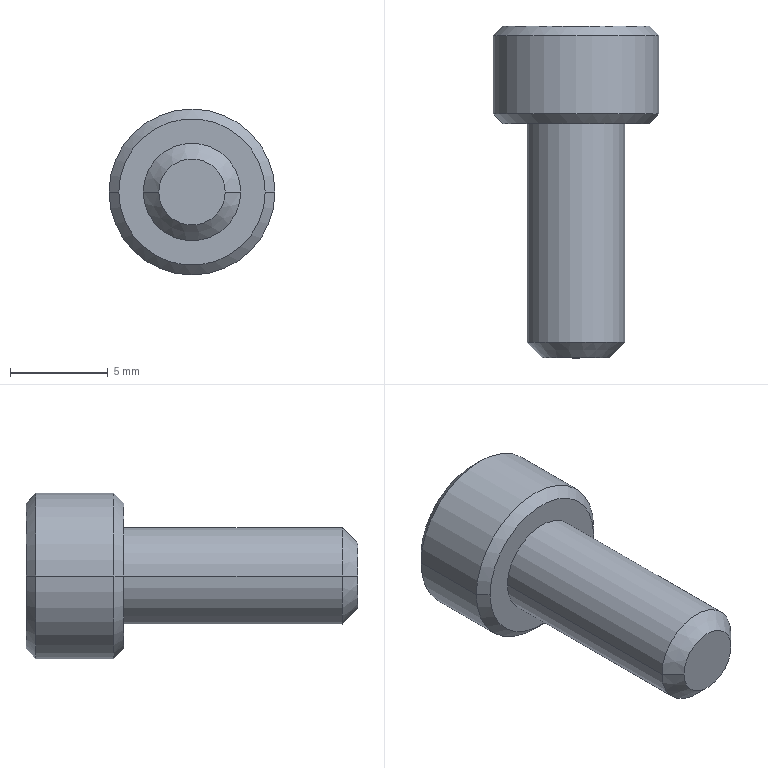Part | STEP file | BB62-M5-12L-13 | 1 solid | 27 faces | box 8.5 x 17 x 8.5 mm | volume 467.118 mm3 | plane 15 | cone 8 | cylinder 4 | commonest cylinder face diameters 5 x2 8.5 x2
STEP:
#1=CARTESIAN_POINT('',(0.,1.178,0.));
#2=VERTEX_POINT('',#1);
#3=CARTESIAN_POINT('',(2.29,2.5,0.));
#4=VERTEX_POINT('',#3);
#5=CARTESIAN_POINT('',(0.,1.178,0.));
#6=DIRECTION('',(0.866,0.5,0.));
#7=VECTOR('',#6,1000.);
#8=LINE('',#5,#7);
#9=EDGE_CURVE('',#2,#4,#8,.T.);
#10=ORIENTED_EDGE('',*,*,#9,.F.);
#11=CARTESIAN_POINT('',(-2.29,2.5,0.));
#12=VERTEX_POINT('',#11);
#13=CARTESIAN_POINT('',(0.,1.178,0.));
#14=DIRECTION('',(-0.866,0.5,0.));
#15=VECTOR('',#14,1000.);
#16=LINE('',#13,#15);
#17=EDGE_CURVE('',#2,#12,#16,.T.);
#18=ORIENTED_EDGE('',*,*,#17,.T.);
#19=CARTESIAN_POINT('',(-1.983,2.5,1.145));
#20=VERTEX_POINT('',#19);
#21=CARTESIAN_POINT('',(0.,2.5,0.));
#22=DIRECTION('',(0.,-1.,0.));
#23=DIRECTION('',(-1.,0.,0.));
#24=AXIS2_PLACEMENT_3D('',#21,#22,#23);
#25=CIRCLE('',#24,2.29);
#26=EDGE_CURVE('',#20,#12,#25,.T.);
#27=ORIENTED_EDGE('',*,*,#26,.F.);
#28=CARTESIAN_POINT('',(0.,2.5,2.29));
#29=VERTEX_POINT('',#28);
#30=CARTESIAN_POINT('',(0.,2.5,0.));
#31=DIRECTION('',(0.,-1.,0.));
#32=DIRECTION('',(-1.,0.,0.));
#33=AXIS2_PLACEMENT_3D('',#30,#31,#32);
#34=CIRCLE('',#33,2.29);
#35=EDGE_CURVE('',#29,#20,#34,.T.);
#36=ORIENTED_EDGE('',*,*,#35,.F.);
#37=CARTESIAN_POINT('',(1.983,2.5,1.145));
#38=VERTEX_POINT('',#37);
#39=CARTESIAN_POINT('',(0.,2.5,0.));
#40=DIRECTION('',(0.,-1.,0.));
#41=DIRECTION('',(-1.,0.,0.));
#42=AXIS2_PLACEMENT_3D('',#39,#40,#41);
#43=CIRCLE('',#42,2.29);
#44=EDGE_CURVE('',#38,#29,#43,.T.);
#45=ORIENTED_EDGE('',*,*,#44,.F.);
#46=CARTESIAN_POINT('',(0.,2.5,0.));
#47=DIRECTION('',(0.,-1.,0.));
#48=DIRECTION('',(-1.,0.,0.));
#49=AXIS2_PLACEMENT_3D('',#46,#47,#48);
#50=CIRCLE('',#49,2.29);
#51=EDGE_CURVE('',#4,#38,#50,.T.);
#52=ORIENTED_EDGE('',*,*,#51,.F.);
#53=EDGE_LOOP('',(#10,#18,#27,#36,#45,#52));
#54=FACE_OUTER_BOUND('',#53,.T.);
#55=CARTESIAN_POINT('',(0.,1001.178,0.));
#56=DIRECTION('',(0.,1.,0.));
#57=DIRECTION('',(1.,0.,0.));
#58=AXIS2_PLACEMENT_3D('',#55,#56,#57);
#59=CONICAL_SURFACE('',#58,1732.051,1.047);
#60=ADVANCED_FACE('',(#54),#59,.F.);
#61=CARTESIAN_POINT('',(1.7,-12.,0.));
#62=VERTEX_POINT('',#61);
#63=CARTESIAN_POINT('',(-1.7,-12.,0.));
#64=VERTEX_POINT('',#63);
#65=CARTESIAN_POINT('',(0.,-12.,0.));
#66=DIRECTION('',(0.,1.,0.));
#67=DIRECTION('',(1.,0.,0.));
#68=AXIS2_PLACEMENT_3D('',#65,#66,#67);
#69=CIRCLE('',#68,1.7);
#70=EDGE_CURVE('',#62,#64,#69,.T.);
#71=ORIENTED_EDGE('',*,*,#70,.T.);
#72=CARTESIAN_POINT('',(-2.5,-11.2,0.));
#73=VERTEX_POINT('',#72);
#74=CARTESIAN_POINT('',(-1.7,-12.,0.));
#75=DIRECTION('',(-0.7071,0.7071,0.));
#76=VECTOR('',#75,1000.);
#77=LINE('',#74,#76);
#78=EDGE_CURVE('',#64,#73,#77,.T.);
#79=ORIENTED_EDGE('',*,*,#78,.T.);
#80=CARTESIAN_POINT('',(2.5,-11.2,0.));
#81=VERTEX_POINT('',#80);
#82=CARTESIAN_POINT('',(0.,-11.2,0.));
#83=DIRECTION('',(0.,-1.,0.));
#84=DIRECTION('',(-1.,0.,0.));
#85=AXIS2_PLACEMENT_3D('',#82,#83,#84);
#86=CIRCLE('',#85,2.5);
#87=EDGE_CURVE('',#73,#81,#86,.T.);
#88=ORIENTED_EDGE('',*,*,#87,.T.);
#89=CARTESIAN_POINT('',(1.7,-12.,0.));
#90=DIRECTION('',(0.7071,0.7071,0.));
#91=VECTOR('',#90,1000.);
#92=LINE('',#89,#91);
#93=EDGE_CURVE('',#62,#81,#92,.T.);
#94=ORIENTED_EDGE('',*,*,#93,.F.);
#95=EDGE_LOOP('',(#71,#79,#88,#94));
#96=FACE_OUTER_BOUND('',#95,.T.);
#97=CARTESIAN_POINT('',(0.,-12.,0.));
#98=DIRECTION('',(0.,1.,0.));
#99=DIRECTION('',(1.,0.,0.));
#100=AXIS2_PLACEMENT_3D('',#97,#98,#99);
#101=CONICAL_SURFACE('',#100,1.7,0.7854);
#102=ADVANCED_FACE('',(#96),#101,.T.);
#103=ORIENTED_EDGE('',*,*,#87,.F.);
#104=CARTESIAN_POINT('',(-2.5,0.,0.));
#105=VERTEX_POINT('',#104);
#106=CARTESIAN_POINT('',(-2.5,-11.2,0.));
#107=DIRECTION('',(0.,1.,0.));
#108=VECTOR('',#107,1000.);
#109=LINE('',#106,#108);
#110=EDGE_CURVE('',#73,#105,#109,.T.);
#111=ORIENTED_EDGE('',*,*,#110,.T.);
#112=CARTESIAN_POINT('',(2.5,0.,0.));
#113=VERTEX_POINT('',#112);
#114=CARTESIAN_POINT('',(0.,0.,0.));
#115=DIRECTION('',(0.,-1.,0.));
#116=DIRECTION('',(-1.,0.,0.));
#117=AXIS2_PLACEMENT_3D('',#114,#115,#116);
#118=CIRCLE('',#117,2.5);
#119=EDGE_CURVE('',#105,#113,#118,.T.);
#120=ORIENTED_EDGE('',*,*,#119,.T.);
#121=CARTESIAN_POINT('',(2.5,-11.2,0.));
#122=DIRECTION('',(0.,1.,0.));
#123=VECTOR('',#122,1000.);
#124=LINE('',#121,#123);
#125=EDGE_CURVE('',#81,#113,#124,.T.);
#126=ORIENTED_EDGE('',*,*,#125,.F.);
#127=EDGE_LOOP('',(#103,#111,#120,#126));
#128=FACE_OUTER_BOUND('',#127,.T.);
#129=CARTESIAN_POINT('',(0.,-11.2,0.));
#130=DIRECTION('',(0.,1.,0.));
#131=DIRECTION('',(1.,0.,0.));
#132=AXIS2_PLACEMENT_3D('',#129,#130,#131);
#133=CYLINDRICAL_SURFACE('',#132,2.5);
#134=ADVANCED_FACE('',(#128),#133,.T.);
#135=CARTESIAN_POINT('',(-3.75,5.,0.));
#136=VERTEX_POINT('',#135);
#137=CARTESIAN_POINT('',(3.75,5.,0.));
#138=VERTEX_POINT('',#137);
#139=CARTESIAN_POINT('',(0.,5.,0.));
#140=DIRECTION('',(0.,-1.,0.));
#141=DIRECTION('',(-1.,0.,0.));
#142=AXIS2_PLACEMENT_3D('',#139,#140,#141);
#143=CIRCLE('',#142,3.75);
#144=EDGE_CURVE('',#136,#138,#143,.T.);
#145=ORIENTED_EDGE('',*,*,#144,.T.);
#146=CARTESIAN_POINT('',(4.25,4.5,0.));
#147=VERTEX_POINT('',#146);
#148=CARTESIAN_POINT('',(4.25,4.5,0.));
#149=DIRECTION('',(0.7071,-0.7071,0.));
#150=VECTOR('',#149,1000.);
#151=LINE('',#148,#150);
#152=EDGE_CURVE('',#138,#147,#151,.T.);
#153=ORIENTED_EDGE('',*,*,#152,.T.);
#154=CARTESIAN_POINT('',(-4.25,4.5,0.));
#155=VERTEX_POINT('',#154);
#156=CARTESIAN_POINT('',(0.,4.5,0.));
#157=DIRECTION('',(0.,-1.,0.));
#158=DIRECTION('',(-1.,0.,0.));
#159=AXIS2_PLACEMENT_3D('',#156,#157,#158);
#160=CIRCLE('',#159,4.25);
#161=EDGE_CURVE('',#155,#147,#160,.T.);
#162=ORIENTED_EDGE('',*,*,#161,.F.);
#163=CARTESIAN_POINT('',(-4.25,4.5,0.));
#164=DIRECTION('',(-0.7071,-0.7071,0.));
#165=VECTOR('',#164,1000.);
#166=LINE('',#163,#165);
#167=EDGE_CURVE('',#136,#155,#166,.T.);
#168=ORIENTED_EDGE('',*,*,#167,.F.);
#169=EDGE_LOOP('',(#145,#153,#162,#168));
#170=FACE_OUTER_BOUND('',#169,.T.);
#171=CARTESIAN_POINT('',(0.,4.5,0.));
#172=DIRECTION('',(0.,-1.,0.));
#173=DIRECTION('',(-1.,0.,0.));
#174=AXIS2_PLACEMENT_3D('',#171,#172,#173);
#175=CONICAL_SURFACE('',#174,4.25,0.7854);
#176=ADVANCED_FACE('',(#170),#175,.T.);
#177=ORIENTED_EDGE('',*,*,#161,.T.);
#178=CARTESIAN_POINT('',(4.25,0.5,0.));
#179=VERTEX_POINT('',#178);
#180=CARTESIAN_POINT('',(4.25,1.62,0.));
#181=DIRECTION('',(0.,-1.,0.));
#182=VECTOR('',#181,1000.);
#183=LINE('',#180,#182);
#184=EDGE_CURVE('',#147,#179,#183,.T.);
#185=ORIENTED_EDGE('',*,*,#184,.T.);
#186=CARTESIAN_POINT('',(-4.25,0.5,0.));
#187=VERTEX_POINT('',#186);
#188=CARTESIAN_POINT('',(0.,0.5,0.));
#189=DIRECTION('',(0.,-1.,0.));
#190=DIRECTION('',(-1.,0.,0.));
#191=AXIS2_PLACEMENT_3D('',#188,#189,#190);
#192=CIRCLE('',#191,4.25);
#193=EDGE_CURVE('',#187,#179,#192,.T.);
#194=ORIENTED_EDGE('',*,*,#193,.F.);
#195=CARTESIAN_POINT('',(-4.25,1.62,0.));
#196=DIRECTION('',(0.,-1.,0.));
#197=VECTOR('',#196,1000.);
#198=LINE('',#195,#197);
#199=EDGE_CURVE('',#155,#187,#198,.T.);
#200=ORIENTED_EDGE('',*,*,#199,.F.);
#201=EDGE_LOOP('',(#177,#185,#194,#200));
#202=FACE_OUTER_BOUND('',#201,.T.);
#203=CARTESIAN_POINT('',(0.,1.62,0.));
#204=DIRECTION('',(0.,-1.,0.));
#205=DIRECTION('',(-1.,0.,0.));
#206=AXIS2_PLACEMENT_3D('',#203,#204,#205);
#207=CYLINDRICAL_SURFACE('',#206,4.25);
#208=ADVANCED_FACE('',(#202),#207,.T.);
#209=CARTESIAN_POINT('',(-3.75,0.,0.));
#210=VERTEX_POINT('',#209);
#211=CARTESIAN_POINT('',(3.75,0.,0.));
#212=VERTEX_POINT('',#211);
#213=CARTESIAN_POINT('',(0.,0.,0.));
#214=DIRECTION('',(0.,-1.,0.));
#215=DIRECTION('',(-1.,0.,0.));
#216=AXIS2_PLACEMENT_3D('',#213,#214,#215);
#217=CIRCLE('',#216,3.75);
#218=EDGE_CURVE('',#210,#212,#217,.T.);
#219=ORIENTED_EDGE('',*,*,#218,.F.);
#220=CARTESIAN_POINT('',(-3.75,0.,0.));
#221=DIRECTION('',(-0.7071,0.7071,0.));
#222=VECTOR('',#221,1000.);
#223=LINE('',#220,#222);
#224=EDGE_CURVE('',#210,#187,#223,.T.);
#225=ORIENTED_EDGE('',*,*,#224,.T.);
#226=ORIENTED_EDGE('',*,*,#193,.T.);
#227=CARTESIAN_POINT('',(3.75,0.,0.));
#228=DIRECTION('',(0.7071,0.7071,0.));
#229=VECTOR('',#228,1000.);
#230=LINE('',#227,#229);
#231=EDGE_CURVE('',#212,#179,#230,.T.);
#232=ORIENTED_EDGE('',*,*,#231,.F.);
#233=EDGE_LOOP('',(#219,#225,#226,#232));
#234=FACE_OUTER_BOUND('',#233,.T.);
#235=CARTESIAN_POINT('',(0.,0.,0.));
#236=DIRECTION('',(0.,1.,0.));
#237=DIRECTION('',(1.,0.,0.));
#238=AXIS2_PLACEMENT_3D('',#235,#236,#237);
#239=CONICAL_SURFACE('',#238,3.75,0.7854);
#240=ADVANCED_FACE('',(#234),#239,.T.);
#241=ORIENTED_EDGE('',*,*,#144,.F.);
#242=CARTESIAN_POINT('',(0.,5.,0.));
#243=DIRECTION('',(0.,-1.,0.));
#244=DIRECTION('',(-1.,0.,0.));
#245=AXIS2_PLACEMENT_3D('',#242,#243,#244);
#246=CIRCLE('',#245,3.75);
#247=EDGE_CURVE('',#138,#136,#246,.T.);
#248=ORIENTED_EDGE('',*,*,#247,.F.);
#249=EDGE_LOOP('',(#241,#248));
#250=FACE_OUTER_BOUND('',#249,.T.);
#251=CARTESIAN_POINT('',(0.,5.,-2.29));
#252=VERTEX_POINT('',#251);
#253=CARTESIAN_POINT('',(-1.983,5.,-1.145));
#254=VERTEX_POINT('',#253);
#255=CARTESIAN_POINT('',(0.,5.,-2.29));
#256=DIRECTION('',(-0.866,0.,0.5));
#257=VECTOR('',#256,1000.);
#258=LINE('',#255,#257);
#259=EDGE_CURVE('',#252,#254,#258,.T.);
#260=ORIENTED_EDGE('',*,*,#259,.F.);
#261=CARTESIAN_POINT('',(1.983,5.,-1.145));
#262=VERTEX_POINT('',#261);
#263=CARTESIAN_POINT('',(1.983,5.,-1.145));
#264=DIRECTION('',(-0.866,0.,-0.5));
#265=VECTOR('',#264,1000.);
#266=LINE('',#263,#265);
#267=EDGE_CURVE('',#262,#252,#266,.T.);
#268=ORIENTED_EDGE('',*,*,#267,.F.);
#269=CARTESIAN_POINT('',(1.983,5.,1.145));
#270=VERTEX_POINT('',#269);
#271=CARTESIAN_POINT('',(1.983,5.,1.145));
#272=DIRECTION('',(0.,0.,-1.));
#273=VECTOR('',#272,1000.);
#274=LINE('',#271,#273);
#275=EDGE_CURVE('',#270,#262,#274,.T.);
#276=ORIENTED_EDGE('',*,*,#275,.F.);
#277=CARTESIAN_POINT('',(0.,5.,2.29));
#278=VERTEX_POINT('',#277);
#279=CARTESIAN_POINT('',(0.,5.,2.29));
#280=DIRECTION('',(0.866,0.,-0.5));
#281=VECTOR('',#280,1000.);
#282=LINE('',#279,#281);
#283=EDGE_CURVE('',#278,#270,#282,.T.);
#284=ORIENTED_EDGE('',*,*,#283,.F.);
#285=CARTESIAN_POINT('',(-1.983,5.,1.145));
#286=VERTEX_POINT('',#285);
#287=CARTESIAN_POINT('',(-1.983,5.,1.145));
#288=DIRECTION('',(0.866,0.,0.5));
#289=VECTOR('',#288,1000.);
#290=LINE('',#287,#289);
#291=EDGE_CURVE('',#286,#278,#290,.T.);
#292=ORIENTED_EDGE('',*,*,#291,.F.);
#293=CARTESIAN_POINT('',(-1.983,5.,-1.145));
#294=DIRECTION('',(0.,0.,1.));
#295=VECTOR('',#294,1000.);
#296=LINE('',#293,#295);
#297=EDGE_CURVE('',#254,#286,#296,.T.);
#298=ORIENTED_EDGE('',*,*,#297,.F.);
#299=EDGE_LOOP('',(#260,#268,#276,#284,#292,#298));
#300=FACE_BOUND('',#299,.T.);
#301=CARTESIAN_POINT('',(3.75,5.,0.));
#302=DIRECTION('',(0.,1.,0.));
#303=DIRECTION('',(1.,0.,0.));
#304=AXIS2_PLACEMENT_3D('',#301,#302,#303);
#305=PLANE('',#304);
#306=ADVANCED_FACE('',(#250,#300),#305,.T.);
#307=CARTESIAN_POINT('',(0.,0.,0.));
#308=DIRECTION('',(0.,-1.,0.));
#309=DIRECTION('',(-1.,0.,0.));
#310=AXIS2_PLACEMENT_3D('',#307,#308,#309);
#311=CIRCLE('',#310,2.5);
#312=EDGE_CURVE('',#113,#105,#311,.T.);
#313=ORIENTED_EDGE('',*,*,#312,.F.);
#314=ORIENTED_EDGE('',*,*,#119,.F.);
#315=EDGE_LOOP('',(#313,#314));
#316=FACE_BOUND('',#315,.T.);
#317=CARTESIAN_POINT('',(0.,0.,0.));
#318=DIRECTION('',(0.,-1.,0.));
#319=DIRECTION('',(-1.,0.,0.));
#320=AXIS2_PLACEMENT_3D('',#317,#318,#319);
#321=CIRCLE('',#320,3.75);
#322=EDGE_CURVE('',#212,#210,#321,.T.);
#323=ORIENTED_EDGE('',*,*,#322,.T.);
#324=ORIENTED_EDGE('',*,*,#218,.T.);
#325=EDGE_LOOP('',(#323,#324));
#326=FACE_OUTER_BOUND('',#325,.T.);
#327=CARTESIAN_POINT('',(0.,0.,0.));
#328=DIRECTION('',(0.,-1.,0.));
#329=DIRECTION('',(-1.,0.,0.));
#330=AXIS2_PLACEMENT_3D('',#327,#328,#329);
#331=PLANE('',#330);
#332=ADVANCED_FACE('',(#316,#326),#331,.T.);
#333=ORIENTED_EDGE('',*,*,#224,.F.);
#334=ORIENTED_EDGE('',*,*,#322,.F.);
#335=ORIENTED_EDGE('',*,*,#231,.T.);
#336=CARTESIAN_POINT('',(0.,0.5,0.));
#337=DIRECTION('',(0.,-1.,0.));
#338=DIRECTION('',(-1.,0.,0.));
#339=AXIS2_PLACEMENT_3D('',#336,#337,#338);
#340=CIRCLE('',#339,4.25);
#341=EDGE_CURVE('',#179,#187,#340,.T.);
#342=ORIENTED_EDGE('',*,*,#341,.T.);
#343=EDGE_LOOP('',(#333,#334,#335,#342));
#344=FACE_OUTER_BOUND('',#343,.T.);
#345=CARTESIAN_POINT('',(0.,0.,0.));
#346=DIRECTION('',(0.,1.,0.));
#347=DIRECTION('',(1.,0.,0.));
#348=AXIS2_PLACEMENT_3D('',#345,#346,#347);
#349=CONICAL_SURFACE('',#348,3.75,0.7854);
#350=ADVANCED_FACE('',(#344),#349,.T.);
#351=ORIENTED_EDGE('',*,*,#184,.F.);
#352=CARTESIAN_POINT('',(0.,4.5,0.));
#353=DIRECTION('',(0.,-1.,0.));
#354=DIRECTION('',(-1.,0.,0.));
#355=AXIS2_PLACEMENT_3D('',#352,#353,#354);
#356=CIRCLE('',#355,4.25);
#357=EDGE_CURVE('',#147,#155,#356,.T.);
#358=ORIENTED_EDGE('',*,*,#357,.T.);
#359=ORIENTED_EDGE('',*,*,#199,.T.);
#360=ORIENTED_EDGE('',*,*,#341,.F.);
#361=EDGE_LOOP('',(#351,#358,#359,#360));
#362=FACE_OUTER_BOUND('',#361,.T.);
#363=CARTESIAN_POINT('',(0.,1.62,0.));
#364=DIRECTION('',(0.,-1.,0.));
#365=DIRECTION('',(-1.,0.,0.));
#366=AXIS2_PLACEMENT_3D('',#363,#364,#365);
#367=CYLINDRICAL_SURFACE('',#366,4.25);
#368=ADVANCED_FACE('',(#362),#367,.T.);
#369=ORIENTED_EDGE('',*,*,#152,.F.);
#370=ORIENTED_EDGE('',*,*,#247,.T.);
#371=ORIENTED_EDGE('',*,*,#167,.T.);
#372=ORIENTED_EDGE('',*,*,#357,.F.);
#373=EDGE_LOOP('',(#369,#370,#371,#372));
#374=FACE_OUTER_BOUND('',#373,.T.);
#375=CARTESIAN_POINT('',(0.,4.5,0.));
#376=DIRECTION('',(0.,-1.,0.));
#377=DIRECTION('',(-1.,0.,0.));
#378=AXIS2_PLACEMENT_3D('',#375,#376,#377);
#379=CONICAL_SURFACE('',#378,4.25,0.7854);
#380=ADVANCED_FACE('',(#374),#379,.T.);
#381=ORIENTED_EDGE('',*,*,#110,.F.);
#382=CARTESIAN_POINT('',(0.,-11.2,0.));
#383=DIRECTION('',(0.,-1.,0.));
#384=DIRECTION('',(-1.,0.,0.));
#385=AXIS2_PLACEMENT_3D('',#382,#383,#384);
#386=CIRCLE('',#385,2.5);
#387=EDGE_CURVE('',#81,#73,#386,.T.);
#388=ORIENTED_EDGE('',*,*,#387,.F.);
#389=ORIENTED_EDGE('',*,*,#125,.T.);
#390=ORIENTED_EDGE('',*,*,#312,.T.);
#391=EDGE_LOOP('',(#381,#388,#389,#390));
#392=FACE_OUTER_BOUND('',#391,.T.);
#393=CARTESIAN_POINT('',(0.,-11.2,0.));
#394=DIRECTION('',(0.,1.,0.));
#395=DIRECTION('',(1.,0.,0.));
#396=AXIS2_PLACEMENT_3D('',#393,#394,#395);
#397=CYLINDRICAL_SURFACE('',#396,2.5);
#398=ADVANCED_FACE('',(#392),#397,.T.);
#399=ORIENTED_EDGE('',*,*,#70,.F.);
#400=CARTESIAN_POINT('',(0.,-12.,0.));
#401=DIRECTION('',(0.,1.,0.));
#402=DIRECTION('',(1.,0.,0.));
#403=AXIS2_PLACEMENT_3D('',#400,#401,#402);
#404=CIRCLE('',#403,1.7);
#405=EDGE_CURVE('',#64,#62,#404,.T.);
#406=ORIENTED_EDGE('',*,*,#405,.F.);
#407=EDGE_LOOP('',(#399,#406));
#408=FACE_OUTER_BOUND('',#407,.T.);
#409=CARTESIAN_POINT('',(0.,-12.,0.));
#410=DIRECTION('',(0.,-1.,0.));
#411=DIRECTION('',(-1.,0.,0.));
#412=AXIS2_PLACEMENT_3D('',#409,#410,#411);
#413=PLANE('',#412);
#414=ADVANCED_FACE('',(#408),#413,.T.);
#415=ORIENTED_EDGE('',*,*,#78,.F.);
#416=ORIENTED_EDGE('',*,*,#405,.T.);
#417=ORIENTED_EDGE('',*,*,#93,.T.);
#418=ORIENTED_EDGE('',*,*,#387,.T.);
#419=EDGE_LOOP('',(#415,#416,#417,#418));
#420=FACE_OUTER_BOUND('',#419,.T.);
#421=CARTESIAN_POINT('',(0.,-12.,0.));
#422=DIRECTION('',(0.,1.,0.));
#423=DIRECTION('',(1.,0.,0.));
#424=AXIS2_PLACEMENT_3D('',#421,#422,#423);
#425=CONICAL_SURFACE('',#424,1.7,0.7854);
#426=ADVANCED_FACE('',(#420),#425,.T.);
#427=CARTESIAN_POINT('',(1.983,2.5,-1.145));
#428=VERTEX_POINT('',#427);
#429=CARTESIAN_POINT('',(0.,2.5,-2.29));
#430=VERTEX_POINT('',#429);
#431=CARTESIAN_POINT('',(1.983,2.5,-1.145));
#432=DIRECTION('',(-0.866,0.,-0.5));
#433=VECTOR('',#432,1000.);
#434=LINE('',#431,#433);
#435=EDGE_CURVE('',#428,#430,#434,.T.);
#436=ORIENTED_EDGE('',*,*,#435,.F.);
#437=CARTESIAN_POINT('',(1.983,5.,-1.145));
#438=DIRECTION('',(0.,-1.,0.));
#439=VECTOR('',#438,1000.);
#440=LINE('',#437,#439);
#441=EDGE_CURVE('',#262,#428,#440,.T.);
#442=ORIENTED_EDGE('',*,*,#441,.F.);
#443=ORIENTED_EDGE('',*,*,#267,.T.);
#444=CARTESIAN_POINT('',(0.,5.,-2.29));
#445=DIRECTION('',(0.,-1.,0.));
#446=VECTOR('',#445,1000.);
#447=LINE('',#444,#446);
#448=EDGE_CURVE('',#252,#430,#447,.T.);
#449=ORIENTED_EDGE('',*,*,#448,.T.);
#450=EDGE_LOOP('',(#436,#442,#443,#449));
#451=FACE_OUTER_BOUND('',#450,.T.);
#452=CARTESIAN_POINT('',(1.983,5.,-1.145));
#453=DIRECTION('',(-0.5,0.,0.866));
#454=DIRECTION('',(0.866,0.,0.5));
#455=AXIS2_PLACEMENT_3D('',#452,#453,#454);
#456=PLANE('',#455);
#457=ADVANCED_FACE('',(#451),#456,.T.);
#458=CARTESIAN_POINT('',(-1.983,2.5,-1.145));
#459=VERTEX_POINT('',#458);
#460=CARTESIAN_POINT('',(0.,2.5,-2.29));
#461=DIRECTION('',(-0.866,0.,0.5));
#462=VECTOR('',#461,1000.);
#463=LINE('',#460,#462);
#464=EDGE_CURVE('',#430,#459,#463,.T.);
#465=ORIENTED_EDGE('',*,*,#464,.F.);
#466=ORIENTED_EDGE('',*,*,#448,.F.);
#467=ORIENTED_EDGE('',*,*,#259,.T.);
#468=CARTESIAN_POINT('',(-1.983,5.,-1.145));
#469=DIRECTION('',(0.,-1.,0.));
#470=VECTOR('',#469,1000.);
#471=LINE('',#468,#470);
#472=EDGE_CURVE('',#254,#459,#471,.T.);
#473=ORIENTED_EDGE('',*,*,#472,.T.);
#474=EDGE_LOOP('',(#465,#466,#467,#473));
#475=FACE_OUTER_BOUND('',#474,.T.);
#476=CARTESIAN_POINT('',(0.,5.,-2.29));
#477=DIRECTION('',(0.5,0.,0.866));
#478=DIRECTION('',(0.866,0.,-0.5));
#479=AXIS2_PLACEMENT_3D('',#476,#477,#478);
#480=PLANE('',#479);
#481=ADVANCED_FACE('',(#475),#480,.T.);
#482=CARTESIAN_POINT('',(-1.983,2.5,-1.145));
#483=DIRECTION('',(0.,0.,1.));
#484=VECTOR('',#483,1000.);
#485=LINE('',#482,#484);
#486=EDGE_CURVE('',#459,#20,#485,.T.);
#487=ORIENTED_EDGE('',*,*,#486,.F.);
#488=ORIENTED_EDGE('',*,*,#472,.F.);
#489=ORIENTED_EDGE('',*,*,#297,.T.);
#490=CARTESIAN_POINT('',(-1.983,5.,1.145));
#491=DIRECTION('',(0.,-1.,0.));
#492=VECTOR('',#491,1000.);
#493=LINE('',#490,#492);
#494=EDGE_CURVE('',#286,#20,#493,.T.);
#495=ORIENTED_EDGE('',*,*,#494,.T.);
#496=EDGE_LOOP('',(#487,#488,#489,#495));
#497=FACE_OUTER_BOUND('',#496,.T.);
#498=CARTESIAN_POINT('',(-1.983,5.,-1.145));
#499=DIRECTION('',(1.,0.,0.));
#500=DIRECTION('',(0.,0.,-1.));
#501=AXIS2_PLACEMENT_3D('',#498,#499,#500);
#502=PLANE('',#501);
#503=ADVANCED_FACE('',(#497),#502,.T.);
#504=CARTESIAN_POINT('',(-1.983,2.5,1.145));
#505=DIRECTION('',(0.866,0.,0.5));
#506=VECTOR('',#505,1000.);
#507=LINE('',#504,#506);
#508=EDGE_CURVE('',#20,#29,#507,.T.);
#509=ORIENTED_EDGE('',*,*,#508,.F.);
#510=ORIENTED_EDGE('',*,*,#494,.F.);
#511=ORIENTED_EDGE('',*,*,#291,.T.);
#512=CARTESIAN_POINT('',(0.,5.,2.29));
#513=DIRECTION('',(0.,-1.,0.));
#514=VECTOR('',#513,1000.);
#515=LINE('',#512,#514);
#516=EDGE_CURVE('',#278,#29,#515,.T.);
#517=ORIENTED_EDGE('',*,*,#516,.T.);
#518=EDGE_LOOP('',(#509,#510,#511,#517));
#519=FACE_OUTER_BOUND('',#518,.T.);
#520=CARTESIAN_POINT('',(-1.983,5.,1.145));
#521=DIRECTION('',(0.5,0.,-0.866));
#522=DIRECTION('',(-0.866,0.,-0.5));
#523=AXIS2_PLACEMENT_3D('',#520,#521,#522);
#524=PLANE('',#523);
#525=ADVANCED_FACE('',(#519),#524,.T.);
#526=CARTESIAN_POINT('',(0.,2.5,2.29));
#527=DIRECTION('',(0.866,0.,-0.5));
#528=VECTOR('',#527,1000.);
#529=LINE('',#526,#528);
#530=EDGE_CURVE('',#29,#38,#529,.T.);
#531=ORIENTED_EDGE('',*,*,#530,.F.);
#532=ORIENTED_EDGE('',*,*,#516,.F.);
#533=ORIENTED_EDGE('',*,*,#283,.T.);
#534=CARTESIAN_POINT('',(1.983,5.,1.145));
#535=DIRECTION('',(0.,-1.,0.));
#536=VECTOR('',#535,1000.);
#537=LINE('',#534,#536);
#538=EDGE_CURVE('',#270,#38,#537,.T.);
#539=ORIENTED_EDGE('',*,*,#538,.T.);
#540=EDGE_LOOP('',(#531,#532,#533,#539));
#541=FACE_OUTER_BOUND('',#540,.T.);
#542=CARTESIAN_POINT('',(0.,5.,2.29));
#543=DIRECTION('',(-0.5,0.,-0.866));
#544=DIRECTION('',(-0.866,0.,0.5));
#545=AXIS2_PLACEMENT_3D('',#542,#543,#544);
#546=PLANE('',#545);
#547=ADVANCED_FACE('',(#541),#546,.T.);
#548=CARTESIAN_POINT('',(1.983,2.5,1.145));
#549=DIRECTION('',(0.,0.,-1.));
#550=VECTOR('',#549,1000.);
#551=LINE('',#548,#550);
#552=EDGE_CURVE('',#38,#428,#551,.T.);
#553=ORIENTED_EDGE('',*,*,#552,.F.);
#554=ORIENTED_EDGE('',*,*,#538,.F.);
#555=ORIENTED_EDGE('',*,*,#275,.T.);
#556=ORIENTED_EDGE('',*,*,#441,.T.);
#557=EDGE_LOOP('',(#553,#554,#555,#556));
#558=FACE_OUTER_BOUND('',#557,.T.);
#559=CARTESIAN_POINT('',(1.983,5.,1.145));
#560=DIRECTION('',(-1.,0.,0.));
#561=DIRECTION('',(0.,0.,1.));
#562=AXIS2_PLACEMENT_3D('',#559,#560,#561);
#563=PLANE('',#562);
#564=ADVANCED_FACE('',(#558),#563,.T.);
#565=ORIENTED_EDGE('',*,*,#435,.T.);
#566=CARTESIAN_POINT('',(0.,2.5,0.));
#567=DIRECTION('',(0.,-1.,0.));
#568=DIRECTION('',(-1.,0.,0.));
#569=AXIS2_PLACEMENT_3D('',#566,#567,#568);
#570=CIRCLE('',#569,2.29);
#571=EDGE_CURVE('',#430,#428,#570,.T.);
#572=ORIENTED_EDGE('',*,*,#571,.T.);
#573=EDGE_LOOP('',(#565,#572));
#574=FACE_OUTER_BOUND('',#573,.T.);
#575=CARTESIAN_POINT('',(0.,2.5,0.));
#576=DIRECTION('',(0.,1.,0.));
#577=DIRECTION('',(1.,0.,0.));
#578=AXIS2_PLACEMENT_3D('',#575,#576,#577);
#579=PLANE('',#578);
#580=ADVANCED_FACE('',(#574),#579,.F.);
#581=ORIENTED_EDGE('',*,*,#552,.T.);
#582=CARTESIAN_POINT('',(0.,2.5,0.));
#583=DIRECTION('',(0.,-1.,0.));
#584=DIRECTION('',(-1.,0.,0.));
#585=AXIS2_PLACEMENT_3D('',#582,#583,#584);
#586=CIRCLE('',#585,2.29);
#587=EDGE_CURVE('',#428,#4,#586,.T.);
#588=ORIENTED_EDGE('',*,*,#587,.T.);
#589=ORIENTED_EDGE('',*,*,#51,.T.);
#590=EDGE_LOOP('',(#581,#588,#589));
#591=FACE_OUTER_BOUND('',#590,.T.);
#592=CARTESIAN_POINT('',(0.,2.5,0.));
#593=DIRECTION('',(0.,1.,0.));
#594=DIRECTION('',(1.,0.,0.));
#595=AXIS2_PLACEMENT_3D('',#592,#593,#594);
#596=PLANE('',#595);
#597=ADVANCED_FACE('',(#591),#596,.F.);
#598=ORIENTED_EDGE('',*,*,#530,.T.);
#599=ORIENTED_EDGE('',*,*,#44,.T.);
#600=EDGE_LOOP('',(#598,#599));
#601=FACE_OUTER_BOUND('',#600,.T.);
#602=CARTESIAN_POINT('',(0.,2.5,0.));
#603=DIRECTION('',(0.,1.,0.));
#604=DIRECTION('',(1.,0.,0.));
#605=AXIS2_PLACEMENT_3D('',#602,#603,#604);
#606=PLANE('',#605);
#607=ADVANCED_FACE('',(#601),#606,.F.);
#608=ORIENTED_EDGE('',*,*,#508,.T.);
#609=ORIENTED_EDGE('',*,*,#35,.T.);
#610=EDGE_LOOP('',(#608,#609));
#611=FACE_OUTER_BOUND('',#610,.T.);
#612=CARTESIAN_POINT('',(0.,2.5,0.));
#613=DIRECTION('',(0.,1.,0.));
#614=DIRECTION('',(1.,0.,0.));
#615=AXIS2_PLACEMENT_3D('',#612,#613,#614);
#616=PLANE('',#615);
#617=ADVANCED_FACE('',(#611),#616,.F.);
#618=ORIENTED_EDGE('',*,*,#486,.T.);
#619=ORIENTED_EDGE('',*,*,#26,.T.);
#620=CARTESIAN_POINT('',(0.,2.5,0.));
#621=DIRECTION('',(0.,-1.,0.));
#622=DIRECTION('',(-1.,0.,0.));
#623=AXIS2_PLACEMENT_3D('',#620,#621,#622);
#624=CIRCLE('',#623,2.29);
#625=EDGE_CURVE('',#12,#459,#624,.T.);
#626=ORIENTED_EDGE('',*,*,#625,.T.);
#627=EDGE_LOOP('',(#618,#619,#626));
#628=FACE_OUTER_BOUND('',#627,.T.);
#629=CARTESIAN_POINT('',(0.,2.5,0.));
#630=DIRECTION('',(0.,1.,0.));
#631=DIRECTION('',(1.,0.,0.));
#632=AXIS2_PLACEMENT_3D('',#629,#630,#631);
#633=PLANE('',#632);
#634=ADVANCED_FACE('',(#628),#633,.F.);
#635=ORIENTED_EDGE('',*,*,#464,.T.);
#636=CARTESIAN_POINT('',(0.,2.5,0.));
#637=DIRECTION('',(0.,-1.,0.));
#638=DIRECTION('',(-1.,0.,0.));
#639=AXIS2_PLACEMENT_3D('',#636,#637,#638);
#640=CIRCLE('',#639,2.29);
#641=EDGE_CURVE('',#459,#430,#640,.T.);
#642=ORIENTED_EDGE('',*,*,#641,.T.);
#643=EDGE_LOOP('',(#635,#642));
#644=FACE_OUTER_BOUND('',#643,.T.);
#645=CARTESIAN_POINT('',(0.,2.5,0.));
#646=DIRECTION('',(0.,1.,0.));
#647=DIRECTION('',(1.,0.,0.));
#648=AXIS2_PLACEMENT_3D('',#645,#646,#647);
#649=PLANE('',#648);
#650=ADVANCED_FACE('',(#644),#649,.F.);
#651=ORIENTED_EDGE('',*,*,#17,.F.);
#652=ORIENTED_EDGE('',*,*,#9,.T.);
#653=ORIENTED_EDGE('',*,*,#587,.F.);
#654=ORIENTED_EDGE('',*,*,#571,.F.);
#655=ORIENTED_EDGE('',*,*,#641,.F.);
#656=ORIENTED_EDGE('',*,*,#625,.F.);
#657=EDGE_LOOP('',(#651,#652,#653,#654,#655,#656));
#658=FACE_OUTER_BOUND('',#657,.T.);
#659=CARTESIAN_POINT('',(0.,1001.178,0.));
#660=DIRECTION('',(0.,1.,0.));
#661=DIRECTION('',(1.,0.,0.));
#662=AXIS2_PLACEMENT_3D('',#659,#660,#661);
#663=CONICAL_SURFACE('',#662,1732.051,1.047);
#664=ADVANCED_FACE('',(#658),#663,.F.);
#665=CLOSED_SHELL('',(#60,#102,#134,#176,#208,#240,#306,#332,#350,#368,#380,#398,#414,#426,#457,#481,#503,#525,#547,#564,#580,#597,#607,#617,#634,#650,#664));
#666=MANIFOLD_SOLID_BREP('',#665);
#667=CARTESIAN_POINT('',(0.,0.,0.));
#668=DIRECTION('',(0.,0.,1.));
#669=DIRECTION('',(1.,0.,0.));
#670=AXIS2_PLACEMENT_3D('',#667,#668,#669);
#671=(LENGTH_UNIT()NAMED_UNIT(*)SI_UNIT(.MILLI.,.METRE.));
#672=UNCERTAINTY_MEASURE_WITH_UNIT(LENGTH_MEASURE(0.00001),#671,'','');
#673=(NAMED_UNIT(*)PLANE_ANGLE_UNIT()SI_UNIT($,.RADIAN.));
#674=(NAMED_UNIT(*)SI_UNIT($,.STERADIAN.)SOLID_ANGLE_UNIT());
#675=(GEOMETRIC_REPRESENTATION_CONTEXT(3)GLOBAL_UNCERTAINTY_ASSIGNED_CONTEXT((#672))GLOBAL_UNIT_ASSIGNED_CONTEXT((#671,#673,#674))REPRESENTATION_CONTEXT('',''));
#676=ADVANCED_BREP_SHAPE_REPRESENTATION('',(#666,#670),#675);